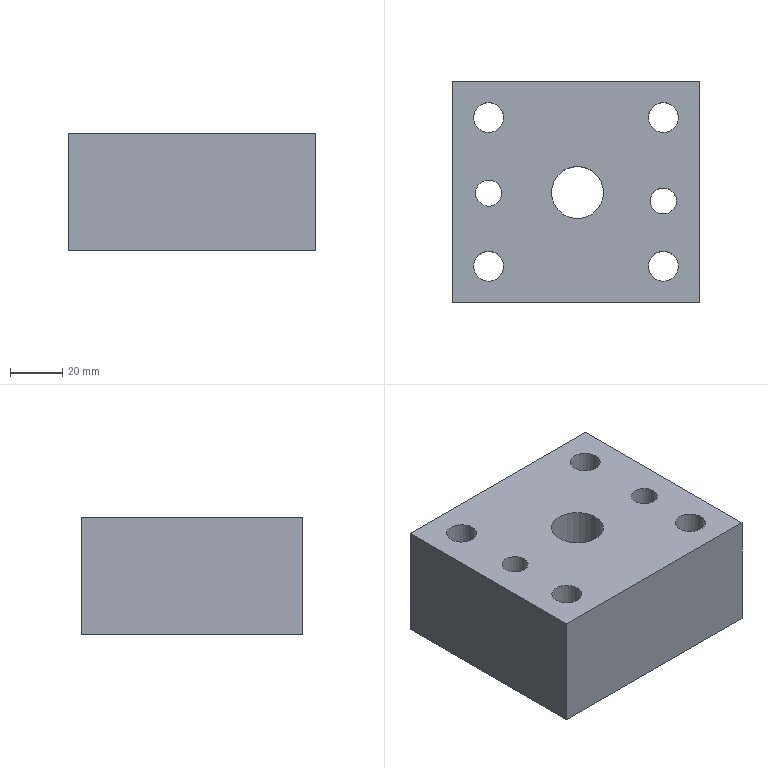Part | STEP file | lll_id4738_x_t | 1 solid | 13 faces | box 95 x 85 x 45 mm | volume 323443 mm3 | cylinder 7 | plane 6 | commonest cylinder face diameters 11.509 x4 10 x2 20 x1
STEP:
#1=CARTESIAN_POINT('',(483.935,342.75,-35.));
#2=VERTEX_POINT('',#1);
#3=CARTESIAN_POINT('',(483.935,342.75,-80.));
#4=VERTEX_POINT('',#3);
#5=CARTESIAN_POINT('',(483.935,342.75,-35.));
#6=DIRECTION('',(0.,0.,-1.));
#7=VECTOR('',#6,1.);
#8=LINE('',#5,#7);
#9=EDGE_CURVE('',#2,#4,#8,.T.);
#10=ORIENTED_EDGE('',*,*,#9,.F.);
#11=CARTESIAN_POINT('',(483.935,257.75,-35.));
#12=VERTEX_POINT('',#11);
#13=CARTESIAN_POINT('',(483.935,310.25,-35.));
#14=DIRECTION('',(0.,1.,0.));
#15=VECTOR('',#14,1.);
#16=LINE('',#13,#15);
#17=EDGE_CURVE('',#12,#2,#16,.T.);
#18=ORIENTED_EDGE('',*,*,#17,.F.);
#19=CARTESIAN_POINT('',(483.935,257.75,-80.));
#20=VERTEX_POINT('',#19);
#21=CARTESIAN_POINT('',(483.935,257.75,-35.));
#22=DIRECTION('',(0.,0.,-1.));
#23=VECTOR('',#22,1.);
#24=LINE('',#21,#23);
#25=EDGE_CURVE('',#12,#20,#24,.T.);
#26=ORIENTED_EDGE('',*,*,#25,.T.);
#27=CARTESIAN_POINT('',(483.935,310.25,-80.));
#28=DIRECTION('',(0.,1.,0.));
#29=VECTOR('',#28,1.);
#30=LINE('',#27,#29);
#31=EDGE_CURVE('',#20,#4,#30,.T.);
#32=ORIENTED_EDGE('',*,*,#31,.T.);
#33=EDGE_LOOP('',(#10,#18,#26,#32));
#34=FACE_OUTER_BOUND('',#33,.T.);
#35=CARTESIAN_POINT('',(483.935,310.25,-35.));
#36=DIRECTION('',(-1.,0.,0.));
#37=DIRECTION('',(0.,1.,0.));
#38=AXIS2_PLACEMENT_3D('',#35,#36,#37);
#39=PLANE('',#38);
#40=ADVANCED_FACE('',(#34),#39,.F.);
#41=ORIENTED_EDGE('',*,*,#25,.F.);
#42=CARTESIAN_POINT('',(388.935,257.75,-35.));
#43=VERTEX_POINT('',#42);
#44=CARTESIAN_POINT('',(466.435,257.75,-35.));
#45=DIRECTION('',(1.,0.,0.));
#46=VECTOR('',#45,1.);
#47=LINE('',#44,#46);
#48=EDGE_CURVE('',#43,#12,#47,.T.);
#49=ORIENTED_EDGE('',*,*,#48,.F.);
#50=CARTESIAN_POINT('',(388.935,257.75,-80.));
#51=VERTEX_POINT('',#50);
#52=CARTESIAN_POINT('',(388.935,257.75,-35.));
#53=DIRECTION('',(0.,0.,-1.));
#54=VECTOR('',#53,1.);
#55=LINE('',#52,#54);
#56=EDGE_CURVE('',#43,#51,#55,.T.);
#57=ORIENTED_EDGE('',*,*,#56,.T.);
#58=CARTESIAN_POINT('',(466.435,257.75,-80.));
#59=DIRECTION('',(1.,0.,0.));
#60=VECTOR('',#59,1.);
#61=LINE('',#58,#60);
#62=EDGE_CURVE('',#51,#20,#61,.T.);
#63=ORIENTED_EDGE('',*,*,#62,.T.);
#64=EDGE_LOOP('',(#41,#49,#57,#63));
#65=FACE_OUTER_BOUND('',#64,.T.);
#66=CARTESIAN_POINT('',(466.435,257.75,-35.));
#67=DIRECTION('',(0.,1.,0.));
#68=DIRECTION('',(1.,0.,0.));
#69=AXIS2_PLACEMENT_3D('',#66,#67,#68);
#70=PLANE('',#69);
#71=ADVANCED_FACE('',(#65),#70,.F.);
#72=ORIENTED_EDGE('',*,*,#56,.F.);
#73=CARTESIAN_POINT('',(388.935,342.75,-35.));
#74=VERTEX_POINT('',#73);
#75=CARTESIAN_POINT('',(388.935,310.25,-35.));
#76=DIRECTION('',(0.,-1.,0.));
#77=VECTOR('',#76,1.);
#78=LINE('',#75,#77);
#79=EDGE_CURVE('',#74,#43,#78,.T.);
#80=ORIENTED_EDGE('',*,*,#79,.F.);
#81=CARTESIAN_POINT('',(388.935,342.75,-80.));
#82=VERTEX_POINT('',#81);
#83=CARTESIAN_POINT('',(388.935,342.75,-35.));
#84=DIRECTION('',(0.,0.,-1.));
#85=VECTOR('',#84,1.);
#86=LINE('',#83,#85);
#87=EDGE_CURVE('',#74,#82,#86,.T.);
#88=ORIENTED_EDGE('',*,*,#87,.T.);
#89=CARTESIAN_POINT('',(388.935,310.25,-80.));
#90=DIRECTION('',(0.,-1.,0.));
#91=VECTOR('',#90,1.);
#92=LINE('',#89,#91);
#93=EDGE_CURVE('',#82,#51,#92,.T.);
#94=ORIENTED_EDGE('',*,*,#93,.T.);
#95=EDGE_LOOP('',(#72,#80,#88,#94));
#96=FACE_OUTER_BOUND('',#95,.T.);
#97=CARTESIAN_POINT('',(388.935,310.25,-35.));
#98=DIRECTION('',(1.,0.,0.));
#99=DIRECTION('',(0.,-1.,0.));
#100=AXIS2_PLACEMENT_3D('',#97,#98,#99);
#101=PLANE('',#100);
#102=ADVANCED_FACE('',(#96),#101,.F.);
#103=CARTESIAN_POINT('',(466.435,342.75,-35.));
#104=DIRECTION('',(-1.,0.,0.));
#105=VECTOR('',#104,1.);
#106=LINE('',#103,#105);
#107=EDGE_CURVE('',#2,#74,#106,.T.);
#108=ORIENTED_EDGE('',*,*,#107,.F.);
#109=ORIENTED_EDGE('',*,*,#9,.T.);
#110=CARTESIAN_POINT('',(466.435,342.75,-80.));
#111=DIRECTION('',(-1.,0.,0.));
#112=VECTOR('',#111,1.);
#113=LINE('',#110,#112);
#114=EDGE_CURVE('',#4,#82,#113,.T.);
#115=ORIENTED_EDGE('',*,*,#114,.T.);
#116=ORIENTED_EDGE('',*,*,#87,.F.);
#117=EDGE_LOOP('',(#108,#109,#115,#116));
#118=FACE_OUTER_BOUND('',#117,.T.);
#119=CARTESIAN_POINT('',(466.435,342.75,-35.));
#120=DIRECTION('',(0.,-1.,0.));
#121=DIRECTION('',(-1.,0.,0.));
#122=AXIS2_PLACEMENT_3D('',#119,#120,#121);
#123=PLANE('',#122);
#124=ADVANCED_FACE('',(#118),#123,.F.);
#125=CARTESIAN_POINT('',(475.69,328.75,-80.));
#126=VERTEX_POINT('',#125);
#127=CARTESIAN_POINT('',(469.935,328.75,-80.));
#128=DIRECTION('',(0.,0.,-1.));
#129=DIRECTION('',(1.,0.,0.));
#130=AXIS2_PLACEMENT_3D('',#127,#128,#129);
#131=CIRCLE('',#130,5.755);
#132=EDGE_CURVE('',#126,#126,#131,.T.);
#133=ORIENTED_EDGE('',*,*,#132,.T.);
#134=EDGE_LOOP('',(#133));
#135=FACE_BOUND('',#134,.T.);
#136=CARTESIAN_POINT('',(475.69,328.75,-35.));
#137=VERTEX_POINT('',#136);
#138=CARTESIAN_POINT('',(469.935,328.75,-35.));
#139=DIRECTION('',(0.,0.,-1.));
#140=DIRECTION('',(1.,0.,0.));
#141=AXIS2_PLACEMENT_3D('',#138,#139,#140);
#142=CIRCLE('',#141,5.755);
#143=EDGE_CURVE('',#137,#137,#142,.T.);
#144=ORIENTED_EDGE('',*,*,#143,.F.);
#145=EDGE_LOOP('',(#144));
#146=FACE_BOUND('',#145,.T.);
#147=CARTESIAN_POINT('',(469.935,328.75,-35.));
#148=DIRECTION('',(0.,0.,-1.));
#149=DIRECTION('',(-1.,0.,0.));
#150=AXIS2_PLACEMENT_3D('',#147,#148,#149);
#151=CYLINDRICAL_SURFACE('',#150,5.755);
#152=ADVANCED_FACE('',(#135,#146),#151,.F.);
#153=CARTESIAN_POINT('',(475.69,271.75,-80.));
#154=VERTEX_POINT('',#153);
#155=CARTESIAN_POINT('',(469.935,271.75,-80.));
#156=DIRECTION('',(0.,0.,-1.));
#157=DIRECTION('',(1.,0.,0.));
#158=AXIS2_PLACEMENT_3D('',#155,#156,#157);
#159=CIRCLE('',#158,5.755);
#160=EDGE_CURVE('',#154,#154,#159,.T.);
#161=ORIENTED_EDGE('',*,*,#160,.T.);
#162=EDGE_LOOP('',(#161));
#163=FACE_BOUND('',#162,.T.);
#164=CARTESIAN_POINT('',(475.69,271.75,-35.));
#165=VERTEX_POINT('',#164);
#166=CARTESIAN_POINT('',(469.935,271.75,-35.));
#167=DIRECTION('',(0.,0.,-1.));
#168=DIRECTION('',(1.,0.,0.));
#169=AXIS2_PLACEMENT_3D('',#166,#167,#168);
#170=CIRCLE('',#169,5.755);
#171=EDGE_CURVE('',#165,#165,#170,.T.);
#172=ORIENTED_EDGE('',*,*,#171,.F.);
#173=EDGE_LOOP('',(#172));
#174=FACE_BOUND('',#173,.T.);
#175=CARTESIAN_POINT('',(469.935,271.75,-35.));
#176=DIRECTION('',(0.,0.,-1.));
#177=DIRECTION('',(-1.,0.,0.));
#178=AXIS2_PLACEMENT_3D('',#175,#176,#177);
#179=CYLINDRICAL_SURFACE('',#178,5.755);
#180=ADVANCED_FACE('',(#163,#174),#179,.F.);
#181=CARTESIAN_POINT('',(474.935,296.75,-80.));
#182=VERTEX_POINT('',#181);
#183=CARTESIAN_POINT('',(469.935,296.75,-80.));
#184=DIRECTION('',(0.,0.,-1.));
#185=DIRECTION('',(1.,0.,0.));
#186=AXIS2_PLACEMENT_3D('',#183,#184,#185);
#187=CIRCLE('',#186,5.);
#188=EDGE_CURVE('',#182,#182,#187,.T.);
#189=ORIENTED_EDGE('',*,*,#188,.T.);
#190=EDGE_LOOP('',(#189));
#191=FACE_BOUND('',#190,.T.);
#192=CARTESIAN_POINT('',(474.935,296.75,-35.));
#193=VERTEX_POINT('',#192);
#194=CARTESIAN_POINT('',(469.935,296.75,-35.));
#195=DIRECTION('',(0.,0.,-1.));
#196=DIRECTION('',(1.,0.,0.));
#197=AXIS2_PLACEMENT_3D('',#194,#195,#196);
#198=CIRCLE('',#197,5.);
#199=EDGE_CURVE('',#193,#193,#198,.T.);
#200=ORIENTED_EDGE('',*,*,#199,.F.);
#201=EDGE_LOOP('',(#200));
#202=FACE_BOUND('',#201,.T.);
#203=CARTESIAN_POINT('',(469.935,296.75,-35.));
#204=DIRECTION('',(0.,0.,-1.));
#205=DIRECTION('',(-1.,0.,0.));
#206=AXIS2_PLACEMENT_3D('',#203,#204,#205);
#207=CYLINDRICAL_SURFACE('',#206,5.);
#208=ADVANCED_FACE('',(#191,#202),#207,.F.);
#209=CARTESIAN_POINT('',(408.69,271.75,-80.));
#210=VERTEX_POINT('',#209);
#211=CARTESIAN_POINT('',(402.935,271.75,-80.));
#212=DIRECTION('',(0.,0.,-1.));
#213=DIRECTION('',(1.,0.,0.));
#214=AXIS2_PLACEMENT_3D('',#211,#212,#213);
#215=CIRCLE('',#214,5.755);
#216=EDGE_CURVE('',#210,#210,#215,.T.);
#217=ORIENTED_EDGE('',*,*,#216,.T.);
#218=EDGE_LOOP('',(#217));
#219=FACE_BOUND('',#218,.T.);
#220=CARTESIAN_POINT('',(408.69,271.75,-35.));
#221=VERTEX_POINT('',#220);
#222=CARTESIAN_POINT('',(402.935,271.75,-35.));
#223=DIRECTION('',(0.,0.,-1.));
#224=DIRECTION('',(1.,0.,0.));
#225=AXIS2_PLACEMENT_3D('',#222,#223,#224);
#226=CIRCLE('',#225,5.755);
#227=EDGE_CURVE('',#221,#221,#226,.T.);
#228=ORIENTED_EDGE('',*,*,#227,.F.);
#229=EDGE_LOOP('',(#228));
#230=FACE_BOUND('',#229,.T.);
#231=CARTESIAN_POINT('',(402.935,271.75,-35.));
#232=DIRECTION('',(0.,0.,-1.));
#233=DIRECTION('',(-1.,0.,0.));
#234=AXIS2_PLACEMENT_3D('',#231,#232,#233);
#235=CYLINDRICAL_SURFACE('',#234,5.755);
#236=ADVANCED_FACE('',(#219,#230),#235,.F.);
#237=CARTESIAN_POINT('',(408.69,328.75,-80.));
#238=VERTEX_POINT('',#237);
#239=CARTESIAN_POINT('',(402.935,328.75,-80.));
#240=DIRECTION('',(0.,0.,-1.));
#241=DIRECTION('',(1.,0.,0.));
#242=AXIS2_PLACEMENT_3D('',#239,#240,#241);
#243=CIRCLE('',#242,5.755);
#244=EDGE_CURVE('',#238,#238,#243,.T.);
#245=ORIENTED_EDGE('',*,*,#244,.T.);
#246=EDGE_LOOP('',(#245));
#247=FACE_BOUND('',#246,.T.);
#248=CARTESIAN_POINT('',(408.69,328.75,-35.));
#249=VERTEX_POINT('',#248);
#250=CARTESIAN_POINT('',(402.935,328.75,-35.));
#251=DIRECTION('',(0.,0.,-1.));
#252=DIRECTION('',(1.,0.,0.));
#253=AXIS2_PLACEMENT_3D('',#250,#251,#252);
#254=CIRCLE('',#253,5.755);
#255=EDGE_CURVE('',#249,#249,#254,.T.);
#256=ORIENTED_EDGE('',*,*,#255,.F.);
#257=EDGE_LOOP('',(#256));
#258=FACE_BOUND('',#257,.T.);
#259=CARTESIAN_POINT('',(402.935,328.75,-35.));
#260=DIRECTION('',(0.,0.,-1.));
#261=DIRECTION('',(-1.,0.,0.));
#262=AXIS2_PLACEMENT_3D('',#259,#260,#261);
#263=CYLINDRICAL_SURFACE('',#262,5.755);
#264=ADVANCED_FACE('',(#247,#258),#263,.F.);
#265=CARTESIAN_POINT('',(407.935,299.75,-80.));
#266=VERTEX_POINT('',#265);
#267=CARTESIAN_POINT('',(402.935,299.75,-80.));
#268=DIRECTION('',(0.,0.,-1.));
#269=DIRECTION('',(1.,0.,0.));
#270=AXIS2_PLACEMENT_3D('',#267,#268,#269);
#271=CIRCLE('',#270,5.);
#272=EDGE_CURVE('',#266,#266,#271,.T.);
#273=ORIENTED_EDGE('',*,*,#272,.T.);
#274=EDGE_LOOP('',(#273));
#275=FACE_BOUND('',#274,.T.);
#276=CARTESIAN_POINT('',(407.935,299.75,-35.));
#277=VERTEX_POINT('',#276);
#278=CARTESIAN_POINT('',(402.935,299.75,-35.));
#279=DIRECTION('',(0.,0.,-1.));
#280=DIRECTION('',(1.,0.,0.));
#281=AXIS2_PLACEMENT_3D('',#278,#279,#280);
#282=CIRCLE('',#281,5.);
#283=EDGE_CURVE('',#277,#277,#282,.T.);
#284=ORIENTED_EDGE('',*,*,#283,.F.);
#285=EDGE_LOOP('',(#284));
#286=FACE_BOUND('',#285,.T.);
#287=CARTESIAN_POINT('',(402.935,299.75,-35.));
#288=DIRECTION('',(0.,0.,-1.));
#289=DIRECTION('',(-1.,0.,0.));
#290=AXIS2_PLACEMENT_3D('',#287,#288,#289);
#291=CYLINDRICAL_SURFACE('',#290,5.);
#292=ADVANCED_FACE('',(#275,#286),#291,.F.);
#293=CARTESIAN_POINT('',(447.,300.,-80.));
#294=VERTEX_POINT('',#293);
#295=CARTESIAN_POINT('',(437.,300.,-80.));
#296=DIRECTION('',(0.,0.,-1.));
#297=DIRECTION('',(1.,0.,0.));
#298=AXIS2_PLACEMENT_3D('',#295,#296,#297);
#299=CIRCLE('',#298,10.);
#300=EDGE_CURVE('',#294,#294,#299,.T.);
#301=ORIENTED_EDGE('',*,*,#300,.T.);
#302=EDGE_LOOP('',(#301));
#303=FACE_BOUND('',#302,.T.);
#304=CARTESIAN_POINT('',(427.,300.,-35.));
#305=VERTEX_POINT('',#304);
#306=CARTESIAN_POINT('',(437.,300.,-35.));
#307=DIRECTION('',(0.,0.,-1.));
#308=DIRECTION('',(-1.,0.,0.));
#309=AXIS2_PLACEMENT_3D('',#306,#307,#308);
#310=CIRCLE('',#309,10.);
#311=EDGE_CURVE('',#305,#305,#310,.T.);
#312=ORIENTED_EDGE('',*,*,#311,.F.);
#313=EDGE_LOOP('',(#312));
#314=FACE_BOUND('',#313,.T.);
#315=CARTESIAN_POINT('',(437.,300.,-35.));
#316=DIRECTION('',(0.,0.,-1.));
#317=DIRECTION('',(-1.,0.,0.));
#318=AXIS2_PLACEMENT_3D('',#315,#316,#317);
#319=CYLINDRICAL_SURFACE('',#318,10.);
#320=ADVANCED_FACE('',(#303,#314),#319,.F.);
#321=ORIENTED_EDGE('',*,*,#93,.F.);
#322=ORIENTED_EDGE('',*,*,#114,.F.);
#323=ORIENTED_EDGE('',*,*,#31,.F.);
#324=ORIENTED_EDGE('',*,*,#62,.F.);
#325=EDGE_LOOP('',(#321,#322,#323,#324));
#326=FACE_BOUND('',#325,.T.);
#327=ORIENTED_EDGE('',*,*,#132,.F.);
#328=EDGE_LOOP('',(#327));
#329=FACE_BOUND('',#328,.T.);
#330=ORIENTED_EDGE('',*,*,#160,.F.);
#331=EDGE_LOOP('',(#330));
#332=FACE_BOUND('',#331,.T.);
#333=ORIENTED_EDGE('',*,*,#188,.F.);
#334=EDGE_LOOP('',(#333));
#335=FACE_BOUND('',#334,.T.);
#336=ORIENTED_EDGE('',*,*,#216,.F.);
#337=EDGE_LOOP('',(#336));
#338=FACE_BOUND('',#337,.T.);
#339=ORIENTED_EDGE('',*,*,#244,.F.);
#340=EDGE_LOOP('',(#339));
#341=FACE_BOUND('',#340,.T.);
#342=ORIENTED_EDGE('',*,*,#272,.F.);
#343=EDGE_LOOP('',(#342));
#344=FACE_BOUND('',#343,.T.);
#345=ORIENTED_EDGE('',*,*,#300,.F.);
#346=EDGE_LOOP('',(#345));
#347=FACE_BOUND('',#346,.T.);
#348=CARTESIAN_POINT('',(2132.435,0.,-80.));
#349=DIRECTION('',(0.,0.,1.));
#350=DIRECTION('',(1.,0.,0.));
#351=AXIS2_PLACEMENT_3D('',#348,#349,#350);
#352=PLANE('',#351);
#353=ADVANCED_FACE('',(#326,#329,#332,#335,#338,#341,#344,#347),#352,.F.);
#354=ORIENTED_EDGE('',*,*,#79,.T.);
#355=ORIENTED_EDGE('',*,*,#48,.T.);
#356=ORIENTED_EDGE('',*,*,#17,.T.);
#357=ORIENTED_EDGE('',*,*,#107,.T.);
#358=EDGE_LOOP('',(#354,#355,#356,#357));
#359=FACE_BOUND('',#358,.T.);
#360=ORIENTED_EDGE('',*,*,#143,.T.);
#361=EDGE_LOOP('',(#360));
#362=FACE_BOUND('',#361,.T.);
#363=ORIENTED_EDGE('',*,*,#171,.T.);
#364=EDGE_LOOP('',(#363));
#365=FACE_BOUND('',#364,.T.);
#366=ORIENTED_EDGE('',*,*,#199,.T.);
#367=EDGE_LOOP('',(#366));
#368=FACE_BOUND('',#367,.T.);
#369=ORIENTED_EDGE('',*,*,#227,.T.);
#370=EDGE_LOOP('',(#369));
#371=FACE_BOUND('',#370,.T.);
#372=ORIENTED_EDGE('',*,*,#255,.T.);
#373=EDGE_LOOP('',(#372));
#374=FACE_BOUND('',#373,.T.);
#375=ORIENTED_EDGE('',*,*,#283,.T.);
#376=EDGE_LOOP('',(#375));
#377=FACE_BOUND('',#376,.T.);
#378=ORIENTED_EDGE('',*,*,#311,.T.);
#379=EDGE_LOOP('',(#378));
#380=FACE_BOUND('',#379,.T.);
#381=CARTESIAN_POINT('',(466.435,325.25,-35.));
#382=DIRECTION('',(0.,0.,-1.));
#383=DIRECTION('',(1.,0.,0.));
#384=AXIS2_PLACEMENT_3D('',#381,#382,#383);
#385=PLANE('',#384);
#386=ADVANCED_FACE('',(#359,#362,#365,#368,#371,#374,#377,#380),#385,.F.);
#387=CLOSED_SHELL('',(#40,#71,#102,#124,#152,#180,#208,#236,#264,#292,#320,#353,#386));
#388=MANIFOLD_SOLID_BREP('',#387);
#389=(LENGTH_UNIT()NAMED_UNIT(*)SI_UNIT(.MILLI.,.METRE.));
#390=UNCERTAINTY_MEASURE_WITH_UNIT(LENGTH_MEASURE(0.00002),#389,'','');
#391=(NAMED_UNIT(*)PLANE_ANGLE_UNIT()SI_UNIT($,.RADIAN.));
#392=PLANE_ANGLE_MEASURE_WITH_UNIT(PLANE_ANGLE_MEASURE(0.01745),#391);
#393=DIMENSIONAL_EXPONENTS(0.,0.,0.,0.,0.,0.,0.);
#394=(CONVERSION_BASED_UNIT('DEGREE',#392)NAMED_UNIT(#393)PLANE_ANGLE_UNIT());
#395=(NAMED_UNIT(*)SI_UNIT($,.STERADIAN.)SOLID_ANGLE_UNIT());
#396=(GEOMETRIC_REPRESENTATION_CONTEXT(3)GLOBAL_UNCERTAINTY_ASSIGNED_CONTEXT((#390))GLOBAL_UNIT_ASSIGNED_CONTEXT((#389,#394,#395))REPRESENTATION_CONTEXT('',''));
#397=ADVANCED_BREP_SHAPE_REPRESENTATION('',(#388),#396);